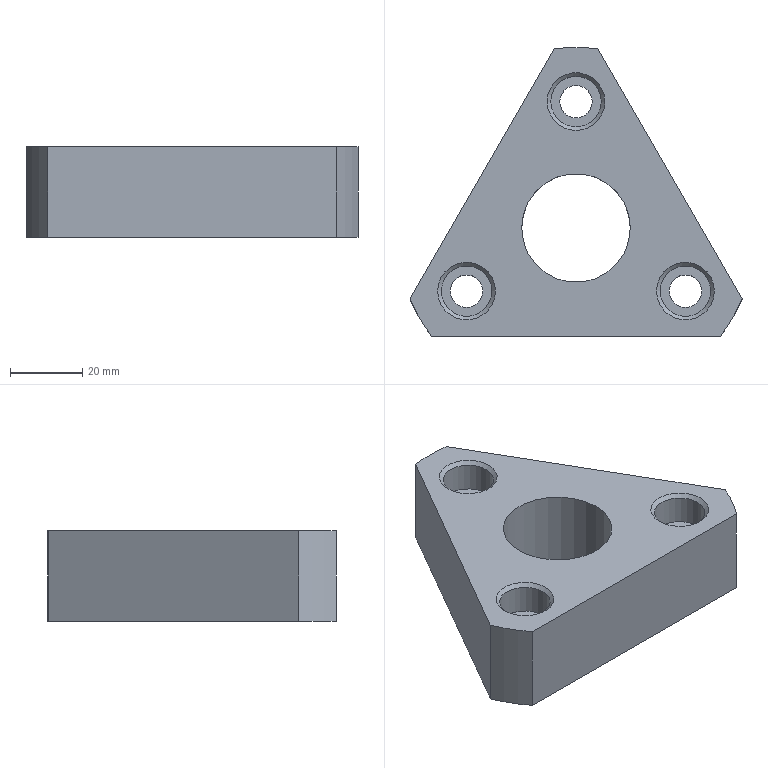NC program | NX | posted with a generic post | part box 91.962 x 80 x 25 mm
Lines 1 to 828 of 11626:
N10 G17 G21 G94 G90
(FLOOR_WALL , TOOL : D50R0.8)
N12 T02 M6
N14 G54
N16 G17 G0 G90 X-78.981 Y42.997 S1200 M3
N18 G43 Z30. H2
N20 Z3.
N22 G94 G1 Z0. F1000.
N24 X-75.981
N26 X75.981
N28 Y20.785
N30 X-75.981
N32 Y-1.428
N34 X75.981
N36 Y-23.64
N38 X-75.981
N40 X-78.981
N42 Z3.
N44 G0 Z30.
N46 M5
(DRILLING , TOOL : ZXZ)
N48 T03 M6
N50 G54
N52 G17 G0 G90 X30.311 Y-27.5 S3000 M3
N54 G43 Z30. H3
N56 G94 G81 G98 Z-1. F250. R3.
N58 X0. Y-10.
N60 Y25.
N62 X-30.311 Y-27.5
N64 G80
N66 G0 X-30.311 Y-27.5 Z30.
N68 M5
(DRILLING_COPY , TOOL : 9.0ZT)
N70 T09 M6
N72 G54
N74 G17 G0 G90 X-30.311 Y-27.5 S1000 M3
N76 G43 Z30. H9
N78 G94 G83 G98 Z-29.204 F200. Q2. R3.
N80 X0. Y25.
N82 X30.311 Y-27.5
N84 G80
N86 G0 X30.311 Y-27.5 Z30.
N88 M5
(DRILLING_COPY_COPY , TOOL : 18.0UZ)
N90 T08 M6
N92 G54
N94 G17 G0 G90 X0. Y-10. S400 M3
N96 G43 Z30. H8
N98 G94 G73 G98 Z-26.5 F100. Q3. R3.
N100 G80
N102 G0 X0. Y-10. Z30.
N104 M5
(ZLEVEL_PROFILE_1 , TOOL : D50R0.8)
N106 T02 M6
N108 G54
N110 G17 G0 G90 X-62.03 Y-7.236 S1197 M3
N112 G43 Z30. H2
N114 Z1.
N116 G94 G1 X-47.719 Y17.551 Z-0.5 F1500.
N118 X-27.719 Y52.192
N120 G2 X-8.969 Y64.564 R25.135
N122 X8.964 Y64.564 R75.101
N124 X27.719 Y52.192 R25.135
N126 G1 X67.719 Y-17.09
N128 G2 X69.064 Y-39.502 R25.102
N130 X60.089 Y-55.051 R75.101
N132 X40. Y-65.101 R25.118
N134 G1 X-40.
N136 G2 X-60.029 Y-55.128 R25.109
N138 G1 X-60.353 Y-54.697
N140 G2 X-69.064 Y-39.502 R75.101
N142 X-67.719 Y-17.09 R25.102
N144 G1 X-47.719 Y17.551
N146 X-47.381 Y18.144 Z-0.512
N148 X-47.044 Y18.736 Z-0.524
N150 X-46.706 Y19.328 Z-0.536
N152 X-46.368 Y19.921 Z-0.548
N154 X-46.029 Y20.513 Z-0.56
N156 X-45.691 Y21.105 Z-0.571
N158 X-45.352 Y21.697 Z-0.583
N160 X-45.014 Y22.289 Z-0.595
N162 X-44.675 Y22.881 Z-0.607
N164 X-44.336 Y23.473 Z-0.619
N166 X-43.997 Y24.065 Z-0.631
N168 X-43.658 Y24.656 Z-0.643
N170 X-43.318 Y25.248 Z-0.655
N172 X-42.979 Y25.84 Z-0.667
N174 X-42.639 Y26.431 Z-0.679
N176 X-42.299 Y27.022 Z-0.69
N178 X-41.96 Y27.614 Z-0.702
N180 X-41.62 Y28.205 Z-0.714
N182 X-41.279 Y28.796 Z-0.726
N184 X-40.939 Y29.387 Z-0.738
N186 X-40.599 Y29.978 Z-0.75
N188 X-40.258 Y30.569 Z-0.762
N190 X-39.918 Y31.16 Z-0.774
N192 X-39.577 Y31.751 Z-0.786
N194 X-39.236 Y32.341 Z-0.798
N196 X-38.895 Y32.932 Z-0.81
N198 X-33.439 Y42.383 Z-1.
N200 X-27.761 Y52.216
N202 G2 X-8.989 Y64.61 R25.15
N204 X8.989 Y64.61 R75.15
N206 X27.761 Y52.216 R25.15
N208 G1 X67.761 Y-17.066
N210 G2 X69.109 Y-39.52 R25.15
N212 X60.12 Y-55.09 R75.15
N214 X40. Y-65.15 R25.15
N216 G1 X-40.
N218 G2 X-60.12 Y-55.09 R25.15
N220 X-69.109 Y-39.52 R75.15
N222 X-67.761 Y-17.066 R25.15
N224 G1 X-47.761 Y17.575
N226 X-33.439 Y42.383 Z-1.5
N228 X-27.761 Y52.216
N230 G2 X-8.989 Y64.61 R25.15
N232 X8.989 Y64.61 R75.15
N234 X27.761 Y52.216 R25.15
N236 G1 X67.761 Y-17.066
N238 G2 X69.109 Y-39.52 R25.15
N240 X60.12 Y-55.09 R75.15
N242 X40. Y-65.15 R25.15
N244 G1 X-40.
N246 G2 X-60.12 Y-55.09 R25.15
N248 X-69.109 Y-39.52 R75.15
N250 X-67.761 Y-17.066 R25.15
N252 G1 X-47.761 Y17.575
N254 X-33.439 Y42.383 Z-2.
N256 X-27.761 Y52.216
N258 G2 X-8.989 Y64.61 R25.15
N260 X8.989 Y64.61 R75.15
N262 X27.761 Y52.216 R25.15
N264 G1 X67.761 Y-17.066
N266 G2 X69.109 Y-39.52 R25.15
N268 X60.12 Y-55.09 R75.15
N270 X40. Y-65.15 R25.15
N272 G1 X-40.
N274 G2 X-60.12 Y-55.09 R25.15
N276 X-69.109 Y-39.52 R75.15
N278 X-67.761 Y-17.066 R25.15
N280 G1 X-47.761 Y17.575
N282 X-33.439 Y42.383 Z-2.5
N284 X-27.761 Y52.216
N286 G2 X-8.989 Y64.61 R25.15
N288 X8.989 Y64.61 R75.15
N290 X27.761 Y52.216 R25.15
N292 G1 X67.761 Y-17.066
N294 G2 X69.109 Y-39.52 R25.15
N296 X60.12 Y-55.09 R75.15
N298 X40. Y-65.15 R25.15
N300 G1 X-40.
N302 G2 X-60.12 Y-55.09 R25.15
N304 X-69.109 Y-39.52 R75.15
N306 X-67.761 Y-17.066 R25.15
N308 G1 X-47.761 Y17.575
N310 X-33.439 Y42.383 Z-3.
N312 X-27.761 Y52.216
N314 G2 X-8.989 Y64.61 R25.15
N316 X8.989 Y64.61 R75.15
N318 X27.761 Y52.216 R25.15
N320 G1 X67.761 Y-17.066
N322 G2 X69.109 Y-39.52 R25.15
N324 X60.12 Y-55.09 R75.15
N326 X40. Y-65.15 R25.15
N328 G1 X-40.
N330 G2 X-60.12 Y-55.09 R25.15
N332 X-69.109 Y-39.52 R75.15
N334 X-67.761 Y-17.066 R25.15
N336 G1 X-47.761 Y17.575
N338 X-33.439 Y42.383 Z-3.5
N340 X-27.761 Y52.216
N342 G2 X-8.989 Y64.61 R25.15
N344 X8.989 Y64.61 R75.15
N346 X27.761 Y52.216 R25.15
N348 G1 X67.761 Y-17.066
N350 G2 X69.109 Y-39.52 R25.15
N352 X60.12 Y-55.09 R75.15
N354 X40. Y-65.15 R25.15
N356 G1 X-40.
N358 G2 X-60.12 Y-55.09 R25.15
N360 X-69.109 Y-39.52 R75.15
N362 X-67.761 Y-17.066 R25.15
N364 G1 X-47.761 Y17.575
N366 X-33.439 Y42.383 Z-4.
N368 X-27.761 Y52.216
N370 G2 X-8.989 Y64.61 R25.15
N372 X8.989 Y64.61 R75.15
N374 X27.761 Y52.216 R25.15
N376 G1 X67.761 Y-17.066
N378 G2 X69.109 Y-39.52 R25.15
N380 X60.12 Y-55.09 R75.15
N382 X40. Y-65.15 R25.15
N384 G1 X-40.
N386 G2 X-60.12 Y-55.09 R25.15
N388 X-69.109 Y-39.52 R75.15
N390 X-67.761 Y-17.066 R25.15
N392 G1 X-47.761 Y17.575
N394 X-33.439 Y42.383 Z-4.5
N396 X-27.761 Y52.216
N398 G2 X-8.989 Y64.61 R25.15
N400 X8.989 Y64.61 R75.15
N402 X27.761 Y52.216 R25.15
N404 G1 X67.761 Y-17.066
N406 G2 X69.109 Y-39.52 R25.15
N408 X60.12 Y-55.09 R75.15
N410 X40. Y-65.15 R25.15
N412 G1 X-40.
N414 G2 X-60.12 Y-55.09 R25.15
N416 X-69.109 Y-39.52 R75.15
N418 X-67.761 Y-17.066 R25.15
N420 G1 X-47.761 Y17.575
N422 X-33.439 Y42.383 Z-5.
N424 X-27.761 Y52.216
N426 G2 X-8.989 Y64.61 R25.15
N428 X8.989 Y64.61 R75.15
N430 X27.761 Y52.216 R25.15
N432 G1 X67.761 Y-17.066
N434 G2 X69.109 Y-39.52 R25.15
N436 X60.12 Y-55.09 R75.15
N438 X40. Y-65.15 R25.15
N440 G1 X-40.
N442 G2 X-60.12 Y-55.09 R25.15
N444 X-69.109 Y-39.52 R75.15
N446 X-67.761 Y-17.066 R25.15
N448 G1 X-47.761 Y17.575
N450 X-33.439 Y42.383 Z-5.5
N452 X-27.761 Y52.216
N454 G2 X-8.989 Y64.61 R25.15
N456 X8.989 Y64.61 R75.15
N458 X27.761 Y52.216 R25.15
N460 G1 X67.761 Y-17.066
N462 G2 X69.109 Y-39.52 R25.15
N464 X60.12 Y-55.09 R75.15
N466 X40. Y-65.15 R25.15
N468 G1 X-40.
N470 G2 X-60.12 Y-55.09 R25.15
N472 X-69.109 Y-39.52 R75.15
N474 X-67.761 Y-17.066 R25.15
N476 G1 X-47.761 Y17.575
N478 X-33.439 Y42.383 Z-6.
N480 X-27.761 Y52.216
N482 G2 X-8.989 Y64.61 R25.15
N484 X8.989 Y64.61 R75.15
N486 X27.761 Y52.216 R25.15
N488 G1 X67.761 Y-17.066
N490 G2 X69.109 Y-39.52 R25.15
N492 X60.12 Y-55.09 R75.15
N494 X40. Y-65.15 R25.15
N496 G1 X-40.
N498 G2 X-60.12 Y-55.09 R25.15
N500 X-69.109 Y-39.52 R75.15
N502 X-67.761 Y-17.066 R25.15
N504 G1 X-47.761 Y17.575
N506 X-33.439 Y42.383 Z-6.5
N508 X-27.761 Y52.216
N510 G2 X-8.989 Y64.61 R25.15
N512 X8.989 Y64.61 R75.15
N514 X27.761 Y52.216 R25.15
N516 G1 X67.761 Y-17.066
N518 G2 X69.109 Y-39.52 R25.15
N520 X60.12 Y-55.09 R75.15
N522 X40. Y-65.15 R25.15
N524 G1 X-40.
N526 G2 X-60.12 Y-55.09 R25.15
N528 X-69.109 Y-39.52 R75.15
N530 X-67.761 Y-17.066 R25.15
N532 G1 X-47.761 Y17.575
N534 X-33.439 Y42.383 Z-7.
N536 X-27.761 Y52.216
N538 G2 X-8.989 Y64.61 R25.15
N540 X8.989 Y64.61 R75.15
N542 X27.761 Y52.216 R25.15
N544 G1 X67.761 Y-17.066
N546 G2 X69.109 Y-39.52 R25.15
N548 X60.12 Y-55.09 R75.15
N550 X40. Y-65.15 R25.15
N552 G1 X-40.
N554 G2 X-60.12 Y-55.09 R25.15
N556 X-69.109 Y-39.52 R75.15
N558 X-67.761 Y-17.066 R25.15
N560 G1 X-47.761 Y17.575
N562 X-33.439 Y42.383 Z-7.5
N564 X-27.761 Y52.216
N566 G2 X-8.989 Y64.61 R25.15
N568 X8.989 Y64.61 R75.15
N570 X27.761 Y52.216 R25.15
N572 G1 X67.761 Y-17.066
N574 G2 X69.109 Y-39.52 R25.15
N576 X60.12 Y-55.09 R75.15
N578 X40. Y-65.15 R25.15
N580 G1 X-40.
N582 G2 X-60.12 Y-55.09 R25.15
N584 X-69.109 Y-39.52 R75.15
N586 X-67.761 Y-17.066 R25.15
N588 G1 X-47.761 Y17.575
N590 X-33.439 Y42.383 Z-8.
N592 X-27.761 Y52.216
N594 G2 X-8.989 Y64.61 R25.15
N596 X8.989 Y64.61 R75.15
N598 X27.761 Y52.216 R25.15
N600 G1 X67.761 Y-17.066
N602 G2 X69.109 Y-39.52 R25.15
N604 X60.12 Y-55.09 R75.15
N606 X40. Y-65.15 R25.15
N608 G1 X-40.
N610 G2 X-60.12 Y-55.09 R25.15
N612 X-69.109 Y-39.52 R75.15
N614 X-67.761 Y-17.066 R25.15
N616 G1 X-47.761 Y17.575
N618 X-33.439 Y42.383 Z-8.5
N620 X-27.761 Y52.216
N622 G2 X-8.989 Y64.61 R25.15
N624 X8.989 Y64.61 R75.15
N626 X27.761 Y52.216 R25.15
N628 G1 X67.761 Y-17.066
N630 G2 X69.109 Y-39.52 R25.15
N632 X60.12 Y-55.09 R75.15
N634 X40. Y-65.15 R25.15
N636 G1 X-40.
N638 G2 X-60.12 Y-55.09 R25.15
N640 X-69.109 Y-39.52 R75.15
N642 X-67.761 Y-17.066 R25.15
N644 G1 X-47.761 Y17.575
N646 X-33.439 Y42.383 Z-9.
N648 X-27.761 Y52.216
N650 G2 X-8.989 Y64.61 R25.15
N652 X8.989 Y64.61 R75.15
N654 X27.761 Y52.216 R25.15
N656 G1 X67.761 Y-17.066
N658 G2 X69.109 Y-39.52 R25.15
N660 X60.12 Y-55.09 R75.15
N662 X40. Y-65.15 R25.15
N664 G1 X-40.
N666 G2 X-60.12 Y-55.09 R25.15
N668 X-69.109 Y-39.52 R75.15
N670 X-67.761 Y-17.066 R25.15
N672 G1 X-47.761 Y17.575
N674 X-33.439 Y42.383 Z-9.5
N676 X-27.761 Y52.216
N678 G2 X-8.989 Y64.61 R25.15
N680 X8.989 Y64.61 R75.15
N682 X27.761 Y52.216 R25.15
N684 G1 X67.761 Y-17.066
N686 G2 X69.109 Y-39.52 R25.15
N688 X60.12 Y-55.09 R75.15
N690 X40. Y-65.15 R25.15
N692 G1 X-40.
N694 G2 X-60.12 Y-55.09 R25.15
N696 X-69.109 Y-39.52 R75.15
N698 X-67.761 Y-17.066 R25.15
N700 G1 X-47.761 Y17.575
N702 X-33.439 Y42.383 Z-10.
N704 X-27.761 Y52.216
N706 G2 X-8.989 Y64.61 R25.15
N708 X8.989 Y64.61 R75.15
N710 X27.761 Y52.216 R25.15
N712 G1 X67.761 Y-17.066
N714 G2 X69.109 Y-39.52 R25.15
N716 X60.12 Y-55.09 R75.15
N718 X40. Y-65.15 R25.15
N720 G1 X-40.
N722 G2 X-60.12 Y-55.09 R25.15
N724 X-69.109 Y-39.52 R75.15
N726 X-67.761 Y-17.066 R25.15
N728 G1 X-47.761 Y17.575
N730 X-33.439 Y42.383 Z-10.5
N732 X-27.761 Y52.216
N734 G2 X-8.989 Y64.61 R25.15
N736 X8.989 Y64.61 R75.15
N738 X27.761 Y52.216 R25.15
N740 G1 X67.761 Y-17.066
N742 G2 X69.109 Y-39.52 R25.15
N744 X60.12 Y-55.09 R75.15
N746 X40. Y-65.15 R25.15
N748 G1 X-40.
N750 G2 X-60.12 Y-55.09 R25.15
N752 X-69.109 Y-39.52 R75.15
N754 X-67.761 Y-17.066 R25.15
N756 G1 X-47.761 Y17.575
N758 X-33.439 Y42.383 Z-11.
N760 X-27.761 Y52.216
N762 G2 X-8.989 Y64.61 R25.15
N764 X8.989 Y64.61 R75.15
N766 X27.761 Y52.216 R25.15
N768 G1 X67.761 Y-17.066
N770 G2 X69.109 Y-39.52 R25.15
N772 X60.12 Y-55.09 R75.15
N774 X40. Y-65.15 R25.15
N776 G1 X-40.
N778 G2 X-60.12 Y-55.09 R25.15
N780 X-69.109 Y-39.52 R75.15
N782 X-67.761 Y-17.066 R25.15
N784 G1 X-47.761 Y17.575
N786 X-33.439 Y42.383 Z-11.5
N788 X-27.761 Y52.216
N790 G2 X-8.989 Y64.61 R25.15
N792 X8.989 Y64.61 R75.15
N794 X27.761 Y52.216 R25.15
N796 G1 X67.761 Y-17.066
N798 G2 X69.109 Y-39.52 R25.15
N800 X60.12 Y-55.09 R75.15
N802 X40. Y-65.15 R25.15
N804 G1 X-40.
N806 G2 X-60.12 Y-55.09 R25.15
N808 X-69.109 Y-39.52 R75.15
N810 X-67.761 Y-17.066 R25.15
N812 G1 X-47.761 Y17.575
N814 X-33.439 Y42.383 Z-12.
N816 X-27.761 Y52.216
N818 G2 X-8.989 Y64.61 R25.15
N820 X8.989 Y64.61 R75.15
N822 X27.761 Y52.216 R25.15
N824 G1 X67.761 Y-17.066
N826 G2 X69.109 Y-39.52 R25.15
N828 X60.12 Y-55.09 R75.15
N830 X40. Y-65.15 R25.15
N832 G1 X-40.
N834 G2 X-60.12 Y-55.09 R25.15
N836 X-69.109 Y-39.52 R75.15
N838 X-67.761 Y-17.066 R25.15
N840 G1 X-47.761 Y17.575
N842 X-33.439 Y42.383 Z-12.5
N844 X-27.761 Y52.216
N846 G2 X-8.989 Y64.61 R25.15
N848 X8.989 Y64.61 R75.15
N850 X27.761 Y52.216 R25.15
N852 G1 X67.761 Y-17.066
N854 G2 X69.109 Y-39.52 R25.15
N856 X60.12 Y-55.09 R75.15
N858 X40. Y-65.15 R25.15
N860 G1 X-40.
N862 G2 X-60.12 Y-55.09 R25.15
N864 X-69.109 Y-39.52 R75.15
N866 X-67.761 Y-17.066 R25.15
N868 G1 X-47.761 Y17.575
N870 X-33.439 Y42.383 Z-13.
N872 X-27.761 Y52.216
N874 G2 X-8.989 Y64.61 R25.15
N876 X8.989 Y64.61 R75.15
N878 X27.761 Y52.216 R25.15
N880 G1 X67.761 Y-17.066
N882 G2 X69.109 Y-39.52 R25.15
N884 X60.12 Y-55.09 R75.15
N886 X40. Y-65.15 R25.15
N888 G1 X-40.
N890 G2 X-60.12 Y-55.09 R25.15
N892 X-69.109 Y-39.52 R75.15
N894 X-67.761 Y-17.066 R25.15
N896 G1 X-47.761 Y17.575
N898 X-33.439 Y42.383 Z-13.5
N900 X-27.761 Y52.216
N902 G2 X-8.989 Y64.61 R25.15
N904 X8.989 Y64.61 R75.15
N906 X27.761 Y52.216 R25.15
N908 G1 X67.761 Y-17.066
N910 G2 X69.109 Y-39.52 R25.15
N912 X60.12 Y-55.09 R75.15
N914 X40. Y-65.15 R25.15
N916 G1 X-40.
N918 G2 X-60.12 Y-55.09 R25.15
N920 X-69.109 Y-39.52 R75.15
N922 X-67.761 Y-17.066 R25.15
N924 G1 X-47.761 Y17.575
N926 X-33.439 Y42.383 Z-14.
N928 X-27.761 Y52.216
N930 G2 X-8.989 Y64.61 R25.15
N932 X8.989 Y64.61 R75.15
N934 X27.761 Y52.216 R25.15
N936 G1 X67.761 Y-17.066
N938 G2 X69.109 Y-39.52 R25.15
N940 X60.12 Y-55.09 R75.15
N942 X40. Y-65.15 R25.15
N944 G1 X-40.
N946 G2 X-60.12 Y-55.09 R25.15
N948 X-69.109 Y-39.52 R75.15
N950 X-67.761 Y-17.066 R25.15
N952 G1 X-47.761 Y17.575
N954 X-33.439 Y42.383 Z-14.5
N956 X-27.761 Y52.216
N958 G2 X-8.989 Y64.61 R25.15
N960 X8.989 Y64.61 R75.15
N962 X27.761 Y52.216 R25.15
N964 G1 X67.761 Y-17.066
N966 G2 X69.109 Y-39.52 R25.15
N968 X60.12 Y-55.09 R75.15
N970 X40. Y-65.15 R25.15
N972 G1 X-40.
N974 G2 X-60.12 Y-55.09 R25.15
N976 X-69.109 Y-39.52 R75.15
N978 X-67.761 Y-17.066 R25.15
N980 G1 X-47.761 Y17.575
N982 X-33.439 Y42.383 Z-15.
N984 X-27.761 Y52.216
N986 G2 X-8.989 Y64.61 R25.15
N988 X8.989 Y64.61 R75.15
N990 X27.761 Y52.216 R25.15
N992 G1 X67.761 Y-17.066
N994 G2 X69.109 Y-39.52 R25.15
N996 X60.12 Y-55.09 R75.15
N998 X40. Y-65.15 R25.15
N1000 G1 X-40.
N1002 G2 X-60.12 Y-55.09 R25.15
N1004 X-69.109 Y-39.52 R75.15
N1006 X-67.761 Y-17.066 R25.15
N1008 G1 X-47.761 Y17.575
N1010 X-33.439 Y42.383 Z-15.5
N1012 X-27.761 Y52.216
N1014 G2 X-8.989 Y64.61 R25.15
N1016 X8.989 Y64.61 R75.15
N1018 X27.761 Y52.216 R25.15
N1020 G1 X67.761 Y-17.066
N1022 G2 X69.109 Y-39.52 R25.15
N1024 X60.12 Y-55.09 R75.15
N1026 X40. Y-65.15 R25.15
N1028 G1 X-40.
N1030 G2 X-60.12 Y-55.09 R25.15
N1032 X-69.109 Y-39.52 R75.15
N1034 X-67.761 Y-17.066 R25.15
N1036 G1 X-47.761 Y17.575
N1038 X-33.439 Y42.383 Z-16.
N1040 X-27.761 Y52.216
N1042 G2 X-8.989 Y64.61 R25.15
N1044 X8.989 Y64.61 R75.15
N1046 X27.761 Y52.216 R25.15
N1048 G1 X67.761 Y-17.066
N1050 G2 X69.109 Y-39.52 R25.15
N1052 X60.12 Y-55.09 R75.15
N1054 X40. Y-65.15 R25.15
N1056 G1 X-40.
N1058 G2 X-60.12 Y-55.09 R25.15
N1060 X-69.109 Y-39.52 R75.15
N1062 X-67.761 Y-17.066 R25.15
N1064 G1 X-47.761 Y17.575
N1066 X-33.439 Y42.383 Z-16.5
N1068 X-27.761 Y52.216
N1070 G2 X-8.989 Y64.61 R25.15
N1072 X8.989 Y64.61 R75.15
N1074 X27.761 Y52.216 R25.15
N1076 G1 X67.761 Y-17.066
N1078 G2 X69.109 Y-39.52 R25.15
N1080 X60.12 Y-55.09 R75.15
N1082 X40. Y-65.15 R25.15
N1084 G1 X-40.
N1086 G2 X-60.12 Y-55.09 R25.15
N1088 X-69.109 Y-39.52 R75.15
N1090 X-67.761 Y-17.066 R25.15
N1092 G1 X-47.761 Y17.575
N1094 X-33.439 Y42.383 Z-17.
N1096 X-27.761 Y52.216
N1098 G2 X-8.989 Y64.61 R25.15
N1100 X8.989 Y64.61 R75.15
N1102 X27.761 Y52.216 R25.15
N1104 G1 X67.761 Y-17.066
N1106 G2 X69.109 Y-39.52 R25.15
N1108 X60.12 Y-55.09 R75.15
N1110 X40. Y-65.15 R25.15
N1112 G1 X-40.
N1114 G2 X-60.12 Y-55.09 R25.15
N1116 X-69.109 Y-39.52 R75.15
N1118 X-67.761 Y-17.066 R25.15
N1120 G1 X-47.761 Y17.575
N1122 X-33.439 Y42.383 Z-17.5
N1124 X-27.761 Y52.216
N1126 G2 X-8.989 Y64.61 R25.15
N1128 X8.989 Y64.61 R75.15
N1130 X27.761 Y52.216 R25.15
N1132 G1 X67.761 Y-17.066
N1134 G2 X69.109 Y-39.52 R25.15
N1136 X60.12 Y-55.09 R75.15
N1138 X40. Y-65.15 R25.15
N1140 G1 X-40.
N1142 G2 X-60.12 Y-55.09 R25.15
N1144 X-69.109 Y-39.52 R75.15
N1146 X-67.761 Y-17.066 R25.15
N1148 G1 X-47.761 Y17.575
N1150 X-33.439 Y42.383 Z-18.
N1152 X-27.761 Y52.216
N1154 G2 X-8.989 Y64.61 R25.15
N1156 X8.989 Y64.61 R75.15
N1158 X27.761 Y52.216 R25.15
N1160 G1 X67.761 Y-17.066
N1162 G2 X69.109 Y-39.52 R25.15
N1164 X60.12 Y-55.09 R75.15
N1166 X40. Y-65.15 R25.15
N1168 G1 X-40.
N1170 G2 X-60.12 Y-55.09 R25.15
N1172 X-69.109 Y-39.52 R75.15
N1174 X-67.761 Y-17.066 R25.15
N1176 G1 X-47.761 Y17.575
N1178 X-33.439 Y42.383 Z-18.5
N1180 X-27.761 Y52.216
N1182 G2 X-8.989 Y64.61 R25.15
N1184 X8.989 Y64.61 R75.15
N1186 X27.761 Y52.216 R25.15
N1188 G1 X67.761 Y-17.066
N1190 G2 X69.109 Y-39.52 R25.15
N1192 X60.12 Y-55.09 R75.15
N1194 X40. Y-65.15 R25.15
N1196 G1 X-40.
N1198 G2 X-60.12 Y-55.09 R25.15
N1200 X-69.109 Y-39.52 R75.15
N1202 X-67.761 Y-17.066 R25.15
N1204 G1 X-47.761 Y17.575
N1206 X-33.439 Y42.383 Z-19.
N1208 X-27.761 Y52.216
N1210 G2 X-8.989 Y64.61 R25.15
N1212 X8.989 Y64.61 R75.15
N1214 X27.761 Y52.216 R25.15
N1216 G1 X67.761 Y-17.066
N1218 G2 X69.109 Y-39.52 R25.15
N1220 X60.12 Y-55.09 R75.15
N1222 X40. Y-65.15 R25.15
N1224 G1 X-40.
N1226 G2 X-60.12 Y-55.09 R25.15
N1228 X-69.109 Y-39.52 R75.15
N1230 X-67.761 Y-17.066 R25.15
N1232 G1 X-47.761 Y17.575
N1234 X-33.439 Y42.383 Z-19.5
N1236 X-27.761 Y52.216
N1238 G2 X-8.989 Y64.61 R25.15
N1240 X8.989 Y64.61 R75.15
N1242 X27.761 Y52.216 R25.15
N1244 G1 X67.761 Y-17.066
N1246 G2 X69.109 Y-39.52 R25.15
N1248 X60.12 Y-55.09 R75.15
N1250 X40. Y-65.15 R25.15
N1252 G1 X-40.
N1254 G2 X-60.12 Y-55.09 R25.15
N1256 X-69.109 Y-39.52 R75.15
N1258 X-67.761 Y-17.066 R25.15
N1260 G1 X-47.761 Y17.575
N1262 X-33.439 Y42.383 Z-20.
N1264 X-27.761 Y52.216
N1266 G2 X-8.989 Y64.61 R25.15
N1268 X8.989 Y64.61 R75.15
N1270 X27.761 Y52.216 R25.15
N1272 G1 X67.761 Y-17.066
N1274 G2 X69.109 Y-39.52 R25.15
N1276 X60.12 Y-55.09 R75.15
N1278 X40. Y-65.15 R25.15
N1280 G1 X-40.
N1282 G2 X-60.12 Y-55.09 R25.15
N1284 X-69.109 Y-39.52 R75.15
N1286 X-67.761 Y-17.066 R25.15
N1288 G1 X-47.761 Y17.575
N1290 X-33.439 Y42.383 Z-20.5
N1292 X-27.761 Y52.216
N1294 G2 X-8.989 Y64.61 R25.15
N1296 X8.989 Y64.61 R75.15
N1298 X27.761 Y52.216 R25.15
N1300 G1 X67.761 Y-17.066
N1302 G2 X69.109 Y-39.52 R25.15
N1304 X60.12 Y-55.09 R75.15
N1306 X40. Y-65.15 R25.15
N1308 G1 X-40.
N1310 G2 X-60.12 Y-55.09 R25.15
N1312 X-69.109 Y-39.52 R75.15
N1314 X-67.761 Y-17.066 R25.15
N1316 G1 X-47.761 Y17.575
N1318 X-33.439 Y42.383 Z-21.
N1320 X-27.761 Y52.216
N1322 G2 X-8.989 Y64.61 R25.15
N1324 X8.989 Y64.61 R75.15
N1326 X27.761 Y52.216 R25.15
N1328 G1 X67.761 Y-17.066
N1330 G2 X69.109 Y-39.52 R25.15
N1332 X60.12 Y-55.09 R75.15
N1334 X40. Y-65.15 R25.15
N1336 G1 X-40.
N1338 G2 X-60.12 Y-55.09 R25.15
N1340 X-69.109 Y-39.52 R75.15
N1342 X-67.761 Y-17.066 R25.15
N1344 G1 X-47.761 Y17.575
N1346 X-33.439 Y42.383 Z-21.5
N1348 X-27.761 Y52.216
N1350 G2 X-8.989 Y64.61 R25.15
N1352 X8.989 Y64.61 R75.15
N1354 X27.761 Y52.216 R25.15
N1356 G1 X67.761 Y-17.066
N1358 G2 X69.109 Y-39.52 R25.15
N1360 X60.12 Y-55.09 R75.15
N1362 X40. Y-65.15 R25.15
N1364 G1 X-40.
N1366 G2 X-60.12 Y-55.09 R25.15
N1368 X-69.109 Y-39.52 R75.15
N1370 X-67.761 Y-17.066 R25.15
N1372 G1 X-47.761 Y17.575
N1374 X-33.439 Y42.383 Z-22.
N1376 X-27.761 Y52.216
N1378 G2 X-8.989 Y64.61 R25.15
N1380 X8.989 Y64.61 R75.15
N1382 X27.761 Y52.216 R25.15
N1384 G1 X67.761 Y-17.066
N1386 G2 X69.109 Y-39.52 R25.15
N1388 X60.12 Y-55.09 R75.15
N1390 X40. Y-65.15 R25.15
N1392 G1 X-40.
N1394 G2 X-60.12 Y-55.09 R25.15
N1396 X-69.109 Y-39.52 R75.15
N1398 X-67.761 Y-17.066 R25.15
N1400 G1 X-47.761 Y17.575
N1402 X-33.439 Y42.383 Z-22.5
N1404 X-27.761 Y52.216
N1406 G2 X-8.989 Y64.61 R25.15
N1408 X8.989 Y64.61 R75.15
N1410 X27.761 Y52.216 R25.15
N1412 G1 X67.761 Y-17.066
N1414 G2 X69.109 Y-39.52 R25.15
N1416 X60.12 Y-55.09 R75.15
N1418 X40. Y-65.15 R25.15
N1420 G1 X-40.
N1422 G2 X-60.12 Y-55.09 R25.15
N1424 X-69.109 Y-39.52 R75.15
N1426 X-67.761 Y-17.066 R25.15
N1428 G1 X-47.761 Y17.575
N1430 X-33.439 Y42.383 Z-23.
N1432 X-27.761 Y52.216
N1434 G2 X-8.989 Y64.61 R25.15
N1436 X8.989 Y64.61 R75.15
N1438 X27.761 Y52.216 R25.15
N1440 G1 X67.761 Y-17.066
N1442 G2 X69.109 Y-39.52 R25.15
N1444 X60.12 Y-55.09 R75.15
N1446 X40. Y-65.15 R25.15
N1448 G1 X-40.
N1450 G2 X-60.12 Y-55.09 R25.15
N1452 X-69.109 Y-39.52 R75.15
N1454 X-67.761 Y-17.066 R25.15
N1456 G1 X-47.761 Y17.575
N1458 X-33.439 Y42.383 Z-23.5
N1460 X-27.761 Y52.216
N1462 G2 X-8.989 Y64.61 R25.15
N1464 X8.989 Y64.61 R75.15
N1466 X27.761 Y52.216 R25.15
N1468 G1 X67.761 Y-17.066
N1470 G2 X69.109 Y-39.52 R25.15
N1472 X60.12 Y-55.09 R75.15
N1474 X40. Y-65.15 R25.15
N1476 G1 X-40.
N1478 G2 X-60.12 Y-55.09 R25.15
N1480 X-69.109 Y-39.52 R75.15
N1482 X-67.761 Y-17.066 R25.15
N1484 G1 X-47.761 Y17.575
N1486 X-33.439 Y42.383 Z-24.
N1488 X-27.761 Y52.216
N1490 G2 X-8.989 Y64.61 R25.15
N1492 X8.989 Y64.61 R75.15
N1494 X27.761 Y52.216 R25.15
N1496 G1 X67.761 Y-17.066
N1498 G2 X69.109 Y-39.52 R25.15
N1500 X60.12 Y-55.09 R75.15
N1502 X40. Y-65.15 R25.15
N1504 G1 X-40.
N1506 G2 X-60.12 Y-55.09 R25.15
N1508 X-69.109 Y-39.52 R75.15
N1510 X-67.761 Y-17.066 R25.15
N1512 G1 X-47.761 Y17.575
N1514 X-33.439 Y42.383 Z-24.5
N1516 X-27.761 Y52.216
N1518 G2 X-8.989 Y64.61 R25.15
N1520 X8.989 Y64.61 R75.15
N1522 X27.761 Y52.216 R25.15
N1524 G1 X67.761 Y-17.066
N1526 G2 X69.109 Y-39.52 R25.15
N1528 X60.12 Y-55.09 R75.15
N1530 X40. Y-65.15 R25.15
N1532 G1 X-40.
N1534 G2 X-60.12 Y-55.09 R25.15
N1536 X-69.109 Y-39.52 R75.15
N1538 X-67.761 Y-17.066 R25.15
N1540 G1 X-47.761 Y17.575
N1542 X-33.439 Y42.383 Z-25.
N1544 X-27.761 Y52.216
N1546 G2 X-8.989 Y64.61 R25.15
N1548 X8.989 Y64.61 R75.15
N1550 X27.761 Y52.216 R25.15
N1552 G1 X67.761 Y-17.066
N1554 G2 X69.109 Y-39.52 R25.15
N1556 X60.12 Y-55.09 R75.15
N1558 X40. Y-65.15 R25.15
N1560 G1 X-40.
N1562 G2 X-60.12 Y-55.09 R25.15
N1564 X-69.109 Y-39.52 R75.15
N1566 X-67.761 Y-17.066 R25.15
N1568 G1 X-47.761 Y17.575
N1570 X-33.439 Y42.383 Z-25.5
N1572 X-27.761 Y52.216
N1574 G2 X-8.989 Y64.61 R25.15
N1576 X8.989 Y64.61 R75.15
N1578 X27.761 Y52.216 R25.15
N1580 G1 X67.761 Y-17.066
N1582 G2 X69.109 Y-39.52 R25.15
N1584 X60.12 Y-55.09 R75.15
N1586 X40. Y-65.15 R25.15
N1588 G1 X-40.
N1590 G2 X-60.12 Y-55.09 R25.15
N1592 X-69.109 Y-39.52 R75.15
N1594 X-67.761 Y-17.066 R25.15
N1596 G1 X-47.761 Y17.575
N1598 X-33.439 Y42.383 Z-26.
N1600 X-27.761 Y52.216
N1602 G2 X-8.989 Y64.61 R25.15
N1604 X8.989 Y64.61 R75.15
N1606 X27.761 Y52.216 R25.15
N1608 G1 X67.761 Y-17.066
N1610 G2 X69.109 Y-39.52 R25.15
N1612 X60.12 Y-55.09 R75.15
N1614 X40. Y-65.15 R25.15
N1616 G1 X-40.
N1618 G2 X-60.12 Y-55.09 R25.15
N1620 X-69.109 Y-39.52 R75.15
N1622 X-67.761 Y-17.066 R25.15
N1624 G1 X-33.439 Y42.383
N1626 Z-25.
N1628 G0 Z30.
N1630 M5